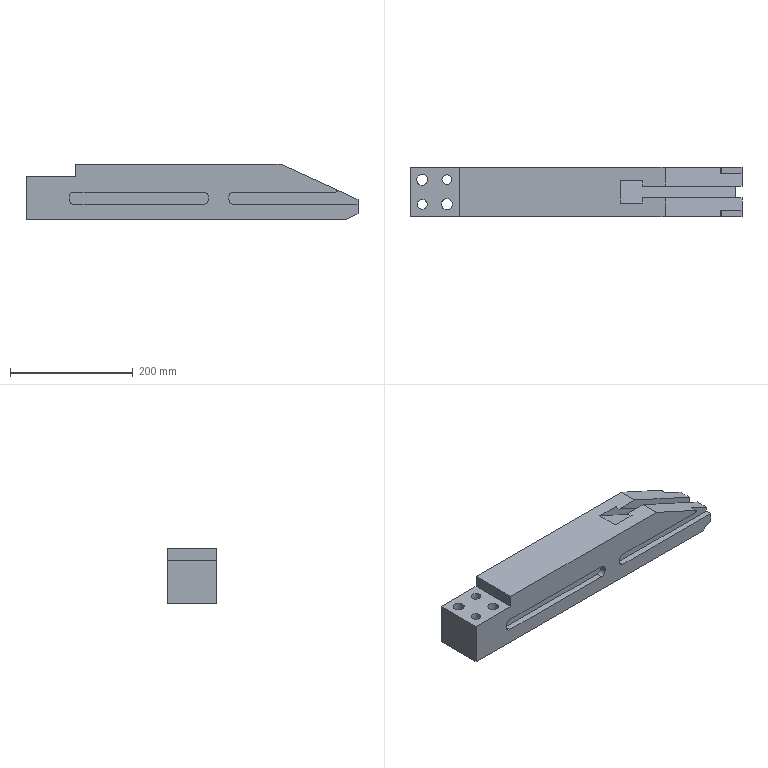Part | STEP file | solid 90 | 1 solid | 59 faces | box 540 x 80 x 90 mm | volume 3073364 mm3 | plane 39 | cylinder 20 | commonest cylinder face diameters 16 x14 4 x2 18 x2 26 x2